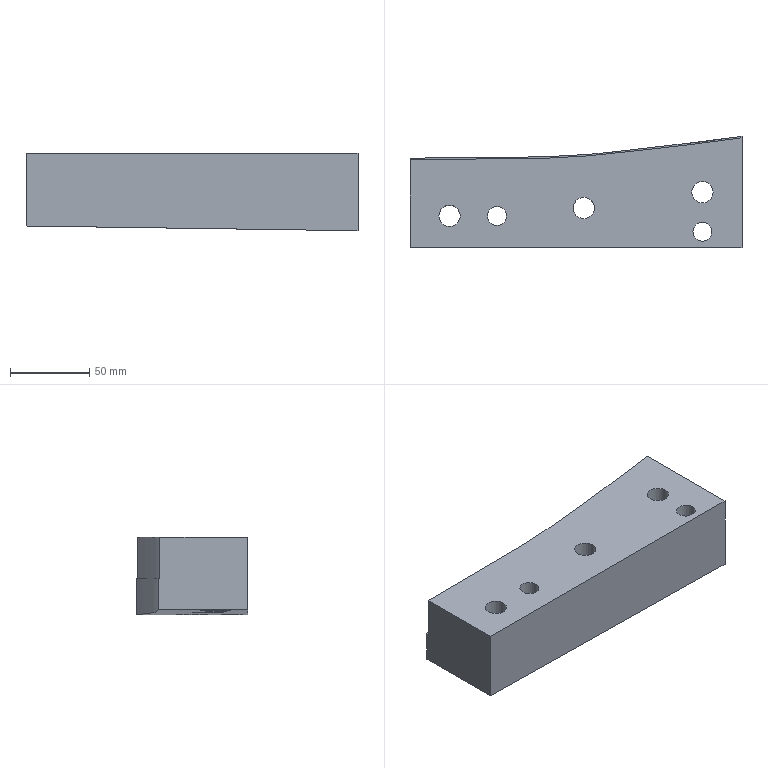Part | NX | features solid 2 | 1 solid | 23 faces | box 210 x 70.368 x 49 mm | volume 559082 mm3 | plane 11 | cylinder 10 | spline 2 | commonest cylinder face diameters 13.5 x3 19.5 x3 12 x2 13 x2
STEP:
#1=CARTESIAN_POINT('',(140.,-80.642,14.));
#2=VERTEX_POINT('',#1);
#3=CARTESIAN_POINT('',(140.,-79.632,14.));
#4=VERTEX_POINT('',#3);
#5=CARTESIAN_POINT('',(140.,-115.282,14.));
#6=DIRECTION('',(0.,1.,0.));
#7=VECTOR('',#6,1000.);
#8=LINE('',#5,#7);
#9=EDGE_CURVE('',#2,#4,#8,.T.);
#10=ORIENTED_EDGE('',*,*,#9,.F.);
#11=CARTESIAN_POINT('',(140.,-80.642,40.));
#12=VERTEX_POINT('',#11);
#13=CARTESIAN_POINT('',(140.,-80.642,57.));
#14=DIRECTION('',(0.,0.,1.));
#15=VECTOR('',#14,1000.);
#16=LINE('',#13,#15);
#17=EDGE_CURVE('',#12,#2,#16,.F.);
#18=ORIENTED_EDGE('',*,*,#17,.F.);
#19=CARTESIAN_POINT('',(140.,-150.,40.));
#20=VERTEX_POINT('',#19);
#21=CARTESIAN_POINT('',(140.,35.09,40.));
#22=DIRECTION('',(0.,1.,0.));
#23=VECTOR('',#22,1000.);
#24=LINE('',#21,#23);
#25=EDGE_CURVE('',#20,#12,#24,.T.);
#26=ORIENTED_EDGE('',*,*,#25,.F.);
#27=CARTESIAN_POINT('',(140.,-150.,-9.));
#28=VERTEX_POINT('',#27);
#29=CARTESIAN_POINT('',(140.,-150.,2.));
#30=DIRECTION('',(0.,0.,-1.));
#31=VECTOR('',#30,1000.);
#32=LINE('',#29,#31);
#33=EDGE_CURVE('',#20,#28,#32,.T.);
#34=ORIENTED_EDGE('',*,*,#33,.T.);
#35=CARTESIAN_POINT('',(140.,-79.632,-9.));
#36=VERTEX_POINT('',#35);
#37=CARTESIAN_POINT('',(140.,-222.,-9.));
#38=DIRECTION('',(0.,-1.,0.));
#39=VECTOR('',#38,1000.);
#40=LINE('',#37,#39);
#41=EDGE_CURVE('',#36,#28,#40,.T.);
#42=ORIENTED_EDGE('',*,*,#41,.F.);
#43=CARTESIAN_POINT('',(140.,-79.632,27.));
#44=DIRECTION('',(0.,0.,-1.));
#45=VECTOR('',#44,1000.);
#46=LINE('',#43,#45);
#47=EDGE_CURVE('',#4,#36,#46,.T.);
#48=ORIENTED_EDGE('',*,*,#47,.F.);
#49=EDGE_LOOP('',(#10,#18,#26,#34,#42,#48));
#50=FACE_BOUND('',#49,.T.);
#51=CARTESIAN_POINT('',(140.,-115.282,21.5));
#52=DIRECTION('',(1.,0.,0.));
#53=DIRECTION('',(0.,0.,-1.));
#54=AXIS2_PLACEMENT_3D('',#51,#52,#53);
#55=PLANE('',#54);
#56=ADVANCED_FACE('',(#50),#55,.T.);
#57=CARTESIAN_POINT('',(-70.,-93.417,14.));
#58=VERTEX_POINT('',#57);
#59=CARTESIAN_POINT('',(-70.,-94.417,14.));
#60=VERTEX_POINT('',#59);
#61=CARTESIAN_POINT('',(-70.,-99.381,14.));
#62=DIRECTION('',(0.,-1.,0.));
#63=VECTOR('',#62,1000.);
#64=LINE('',#61,#63);
#65=EDGE_CURVE('',#58,#60,#64,.T.);
#66=ORIENTED_EDGE('',*,*,#65,.F.);
#67=CARTESIAN_POINT('',(-70.,-93.417,-6.));
#68=VERTEX_POINT('',#67);
#69=CARTESIAN_POINT('',(-70.,-93.417,27.));
#70=DIRECTION('',(0.,0.,-1.));
#71=VECTOR('',#70,1000.);
#72=LINE('',#69,#71);
#73=EDGE_CURVE('',#58,#68,#72,.T.);
#74=ORIENTED_EDGE('',*,*,#73,.T.);
#75=CARTESIAN_POINT('',(-70.,-150.,-6.));
#76=VERTEX_POINT('',#75);
#77=CARTESIAN_POINT('',(-70.,-99.381,-6.));
#78=DIRECTION('',(0.,-1.,0.));
#79=VECTOR('',#78,1000.);
#80=LINE('',#77,#79);
#81=EDGE_CURVE('',#68,#76,#80,.T.);
#82=ORIENTED_EDGE('',*,*,#81,.T.);
#83=CARTESIAN_POINT('',(-70.,-150.,40.));
#84=VERTEX_POINT('',#83);
#85=CARTESIAN_POINT('',(-70.,-150.,-66.));
#86=DIRECTION('',(0.,0.,-1.));
#87=VECTOR('',#86,1000.);
#88=LINE('',#85,#87);
#89=EDGE_CURVE('',#84,#76,#88,.T.);
#90=ORIENTED_EDGE('',*,*,#89,.F.);
#91=CARTESIAN_POINT('',(-70.,-94.417,40.));
#92=VERTEX_POINT('',#91);
#93=CARTESIAN_POINT('',(-70.,35.09,40.));
#94=DIRECTION('',(0.,-1.,0.));
#95=VECTOR('',#94,1000.);
#96=LINE('',#93,#95);
#97=EDGE_CURVE('',#92,#84,#96,.T.);
#98=ORIENTED_EDGE('',*,*,#97,.F.);
#99=CARTESIAN_POINT('',(-70.,-94.417,57.));
#100=DIRECTION('',(0.,0.,1.));
#101=VECTOR('',#100,1000.);
#102=LINE('',#99,#101);
#103=EDGE_CURVE('',#60,#92,#102,.T.);
#104=ORIENTED_EDGE('',*,*,#103,.F.);
#105=EDGE_LOOP('',(#66,#74,#82,#90,#98,#104));
#106=FACE_BOUND('',#105,.T.);
#107=CARTESIAN_POINT('',(-70.,-99.381,-66.));
#108=DIRECTION('',(-1.,0.,0.));
#109=DIRECTION('',(0.,0.,1.));
#110=AXIS2_PLACEMENT_3D('',#107,#108,#109);
#111=PLANE('',#110);
#112=ADVANCED_FACE('',(#106),#111,.T.);
#113=CARTESIAN_POINT('',(-190.231,-121.49,14.));
#114=CARTESIAN_POINT('',(-188.654,-121.152,14.));
#115=CARTESIAN_POINT('',(-185.47,-120.627,14.));
#116=CARTESIAN_POINT('',(-180.656,-120.141,14.));
#117=CARTESIAN_POINT('',(-175.882,-119.326,14.));
#118=CARTESIAN_POINT('',(-169.679,-117.528,14.));
#119=CARTESIAN_POINT('',(-162.185,-114.539,14.));
#120=CARTESIAN_POINT('',(-153.086,-111.254,14.));
#121=CARTESIAN_POINT('',(-144.031,-107.845,14.));
#122=CARTESIAN_POINT('',(-136.465,-105.061,14.));
#123=CARTESIAN_POINT('',(-130.418,-102.814,14.));
#124=CARTESIAN_POINT('',(-125.812,-101.329,14.));
#125=CARTESIAN_POINT('',(-121.306,-99.566,14.));
#126=CARTESIAN_POINT('',(-116.876,-97.626,14.));
#127=CARTESIAN_POINT('',(-112.335,-95.923,14.));
#128=CARTESIAN_POINT('',(-107.564,-95.05,14.));
#129=CARTESIAN_POINT('',(-102.756,-94.525,14.));
#130=CARTESIAN_POINT('',(-96.349,-93.771,14.));
#131=CARTESIAN_POINT('',(-89.902,-93.468,14.));
#132=CARTESIAN_POINT('',(-83.452,-93.448,14.));
#133=CARTESIAN_POINT('',(-77.002,-93.469,14.));
#134=CARTESIAN_POINT('',(-68.939,-93.411,14.));
#135=CARTESIAN_POINT('',(-56.04,-93.3,14.));
#136=CARTESIAN_POINT('',(-33.465,-93.184,14.));
#137=CARTESIAN_POINT('',(-7.666,-93.074,14.));
#138=CARTESIAN_POINT('',(14.907,-92.653,14.));
#139=CARTESIAN_POINT('',(27.794,-92.068,14.));
#140=CARTESIAN_POINT('',(40.668,-91.245,14.));
#141=CARTESIAN_POINT('',(51.917,-90.291,14.));
#142=CARTESIAN_POINT('',(61.528,-89.174,14.));
#143=CARTESIAN_POINT('',(67.939,-88.466,14.));
#144=CARTESIAN_POINT('',(79.125,-86.95,14.));
#145=CARTESIAN_POINT('',(95.161,-85.253,14.));
#146=CARTESIAN_POINT('',(114.404,-83.21,14.));
#147=CARTESIAN_POINT('',(133.568,-80.524,14.));
#148=CARTESIAN_POINT('',(152.734,-77.861,14.));
#149=CARTESIAN_POINT('',(171.916,-75.326,14.));
#150=CARTESIAN_POINT('',(191.055,-72.413,14.));
#151=CARTESIAN_POINT('',(207.17,-71.468,14.));
#152=CARTESIAN_POINT('',(219.951,-69.697,14.));
#153=CARTESIAN_POINT('',(232.724,-67.899,14.));
#154=CARTESIAN_POINT('',(248.708,-65.766,14.));
#155=CARTESIAN_POINT('',(267.87,-63.074,14.));
#156=CARTESIAN_POINT('',(287.038,-60.44,14.));
#157=CARTESIAN_POINT('',(301.448,-58.682,14.));
#158=CARTESIAN_POINT('',(310.976,-56.987,14.));
#159=CARTESIAN_POINT('',(314.916,-56.135,14.));
#160=CARTESIAN_POINT('',(318.052,-55.382,14.));
#161=CARTESIAN_POINT('',(320.39,-54.76,14.));
#162=CARTESIAN_POINT('',(322.686,-53.981,14.));
#163=CARTESIAN_POINT('',(325.595,-52.578,14.));
#164=CARTESIAN_POINT('',(328.769,-50.098,14.));
#165=CARTESIAN_POINT('',(332.247,-46.69,14.));
#166=CARTESIAN_POINT('',(335.795,-43.406,14.));
#167=CARTESIAN_POINT('',(343.661,-37.758,14.));
#168=CARTESIAN_POINT('',(355.164,-28.914,14.));
#169=CARTESIAN_POINT('',(370.422,-17.018,14.));
#170=CARTESIAN_POINT('',(383.264,-7.249,14.));
#171=CARTESIAN_POINT('',(392.416,-0.6713,14.));
#172=CARTESIAN_POINT('',(396.953,2.733,14.));
#173=CARTESIAN_POINT('',(398.886,5.372,14.));
#174=CARTESIAN_POINT('',(399.725,7.654,14.));
#175=CARTESIAN_POINT('',(399.76,10.078,14.));
#176=CARTESIAN_POINT('',(399.483,13.317,14.));
#177=CARTESIAN_POINT('',(399.712,17.34,14.));
#178=CARTESIAN_POINT('',(399.612,22.179,14.));
#179=CARTESIAN_POINT('',(399.633,31.854,14.));
#180=CARTESIAN_POINT('',(399.593,46.366,14.));
#181=CARTESIAN_POINT('',(399.637,62.491,14.));
#182=CARTESIAN_POINT('',(399.588,73.779,14.));
#183=CARTESIAN_POINT('',(399.652,79.422,14.));
#184=CARTESIAN_POINT('',(399.59,82.647,14.));
#185=CARTESIAN_POINT('',(399.564,85.065,14.));
#186=CARTESIAN_POINT('',(399.725,87.486,14.));
#187=CARTESIAN_POINT('',(399.756,89.902,14.));
#188=CARTESIAN_POINT('',(399.247,92.301,14.));
#189=CARTESIAN_POINT('',(397.362,95.008,14.));
#190=CARTESIAN_POINT('',(393.635,96.774,14.));
#191=CARTESIAN_POINT('',(389.279,98.826,14.));
#192=CARTESIAN_POINT('',(384.732,100.498,14.));
#193=CARTESIAN_POINT('',(378.765,102.95,14.));
#194=CARTESIAN_POINT('',(362.589,110.229,14.));
#195=CARTESIAN_POINT('',(344.928,118.135,14.));
#196=CARTESIAN_POINT('',(327.281,126.072,14.));
#197=CARTESIAN_POINT('',(319.932,129.381,14.));
#198=CARTESIAN_POINT('',(314.075,132.102,14.));
#199=CARTESIAN_POINT('',(309.387,133.376,14.));
#200=CARTESIAN_POINT('',(304.547,133.785,14.));
#201=CARTESIAN_POINT('',(299.716,133.401,14.));
#202=CARTESIAN_POINT('',(294.929,132.704,14.));
#203=CARTESIAN_POINT('',(288.543,131.8,14.));
#204=CARTESIAN_POINT('',(277.364,130.241,14.));
#205=CARTESIAN_POINT('',(242.2,125.552,14.));
#206=CARTESIAN_POINT('',(184.637,118.048,14.));
#207=CARTESIAN_POINT('',(120.701,109.541,14.));
#208=CARTESIAN_POINT('',(69.531,102.902,14.));
#209=CARTESIAN_POINT('',(40.777,98.94,14.));
#210=CARTESIAN_POINT('',(21.566,96.615,14.));
#211=CARTESIAN_POINT('',(8.743,95.212,14.));
#212=CARTESIAN_POINT('',(-7.301,93.575,14.));
#213=CARTESIAN_POINT('',(-26.625,92.505,14.));
#214=CARTESIAN_POINT('',(-45.971,92.017,14.));
#215=CARTESIAN_POINT('',(-62.09,91.675,14.));
#216=CARTESIAN_POINT('',(-74.987,91.256,14.));
#217=CARTESIAN_POINT('',(-84.664,91.165,14.));
#218=CARTESIAN_POINT('',(-94.319,91.781,14.));
#219=CARTESIAN_POINT('',(-103.929,92.966,14.));
#220=CARTESIAN_POINT('',(-113.495,94.403,14.));
#221=CARTESIAN_POINT('',(-119.856,95.492,14.));
#222=CARTESIAN_POINT('',(-122.997,96.222,14.));
#223=B_SPLINE_CURVE_WITH_KNOTS('',3,(#113,#114,#115,#116,#117,#118,#119,#120,#121,#122,#123,#124,#125,#126,#127,#128,#129,#130,#131,#132,#133,#134,#135,#136,#137,#138,#139,#140,#141,#142,#143,#144,#145,#146,#147,#148,#149,#150,#151,#152,#153,#154,#155,#156,#157,#158,#159,#160,#161,#162,#163,#164,#165,#166,#167,#168,#169,#170,#171,#172,#173,#174,#175,#176,#177,#178,#179,#180,#181,#182,#183,#184,#185,#186,#187,#188,#189,#190,#191,#192,#193,#194,#195,#196,#197,#198,#199,#200,#201,#202,#203,#204,#205,#206,#207,#208,#209,#210,#211,#212,#213,#214,#215,#216,#217,#218,#219,#220,#221,#222),.UNSPECIFIED.,.F.,.F.,(4,1,1,1,1,1,1,1,1,1,1,1,1,1,1,1,1,1,1,1,1,1,1,1,1,1,1,1,1,1,1,1,1,1,1,1,1,1,1,1,1,1,1,1,1,1,1,1,1,1,1,1,1,1,1,1,1,1,1,1,1,1,1,1,1,1,1,1,1,1,1,1,1,1,1,1,1,1,1,1,1,1,1,1,1,1,1,1,1,1,1,1,1,1,1,1,1,1,1,1,1,1,1,1,1,1,1,4),(0.4704,0.4724,0.4745,0.4766,0.4786,0.4828,0.4869,0.491,0.4952,0.4972,0.4993,0.5014,0.5035,0.5055,0.5076,0.5097,0.5117,0.5159,0.5179,0.52,0.5241,0.5283,0.5366,0.5531,0.5614,0.5655,0.5697,0.5779,0.58,0.5821,0.5862,0.5945,0.6028,0.611,0.6193,0.6276,0.6359,0.6441,0.6483,0.6524,0.6607,0.669,0.6772,0.6855,0.6876,0.6897,0.6907,0.6917,0.6928,0.6938,0.6959,0.6979,0.7,0.7021,0.7103,0.7186,0.7269,0.731,0.7331,0.7341,0.7352,0.7362,0.7372,0.7393,0.7414,0.7435,0.7517,0.76,0.7641,0.7662,0.7672,0.7683,0.7693,0.7703,0.7714,0.7724,0.7745,0.7766,0.7786,0.7807,0.7848,0.8014,0.8055,0.8097,0.8117,0.8138,0.8159,0.8179,0.82,0.8221,0.8262,0.8345,0.8676,0.9007,0.9172,0.9338,0.9379,0.9421,0.9503,0.9586,0.9669,0.9752,0.9793,0.9834,0.9876,0.9917,0.9959,1.),.UNSPECIFIED.);
#224=EDGE_CURVE('',#4,#58,#223,.F.);
#225=ORIENTED_EDGE('',*,*,#224,.F.);
#226=ORIENTED_EDGE('',*,*,#47,.T.);
#227=CARTESIAN_POINT('',(140.,-79.632,-9.));
#228=CARTESIAN_POINT('',(131.311,-80.839,-8.876));
#229=CARTESIAN_POINT('',(113.944,-83.357,-8.628));
#230=CARTESIAN_POINT('',(92.136,-85.521,-8.316));
#231=CARTESIAN_POINT('',(76.894,-87.264,-8.098));
#232=CARTESIAN_POINT('',(68.201,-88.424,-7.974));
#233=CARTESIAN_POINT('',(59.49,-89.412,-7.85));
#234=CARTESIAN_POINT('',(48.597,-90.606,-7.694));
#235=CARTESIAN_POINT('',(31.113,-91.951,-7.444));
#236=CARTESIAN_POINT('',(9.179,-92.893,-7.131));
#237=CARTESIAN_POINT('',(-26.014,-93.171,-6.628));
#238=CARTESIAN_POINT('',(-52.407,-93.281,-6.251));
#239=CARTESIAN_POINT('',(-70.,-93.417,-6.));
#240=B_SPLINE_CURVE_WITH_KNOTS('',3,(#227,#228,#229,#230,#231,#232,#233,#234,#235,#236,#237,#238,#239),.UNSPECIFIED.,.F.,.F.,(4,1,1,1,1,1,1,1,1,1,4),(0.,0.0263,0.0526,0.06575,0.07233,0.0789,0.09205,0.1052,0.1315,0.1578,0.2104),.UNSPECIFIED.);
#241=EDGE_CURVE('',#36,#68,#240,.T.);
#242=ORIENTED_EDGE('',*,*,#241,.T.);
#243=ORIENTED_EDGE('',*,*,#73,.F.);
#244=EDGE_LOOP('',(#225,#226,#242,#243));
#245=FACE_BOUND('',#244,.T.);
#246=CARTESIAN_POINT('',(-70.,-93.417,14.));
#247=CARTESIAN_POINT('',(-70.,-93.417,-9.138));
#248=CARTESIAN_POINT('',(-52.44,-93.282,14.));
#249=CARTESIAN_POINT('',(-52.44,-93.282,-9.138));
#250=CARTESIAN_POINT('',(-26.1,-93.171,14.));
#251=CARTESIAN_POINT('',(-26.1,-93.171,-9.138));
#252=CARTESIAN_POINT('',(9.024,-92.895,14.));
#253=CARTESIAN_POINT('',(9.024,-92.895,-9.138));
#254=CARTESIAN_POINT('',(30.956,-91.96,14.));
#255=CARTESIAN_POINT('',(30.956,-91.96,-9.138));
#256=CARTESIAN_POINT('',(48.469,-90.618,14.));
#257=CARTESIAN_POINT('',(48.469,-90.618,-9.138));
#258=CARTESIAN_POINT('',(59.38,-89.424,14.));
#259=CARTESIAN_POINT('',(59.38,-89.424,-9.138));
#260=CARTESIAN_POINT('',(68.104,-88.436,14.));
#261=CARTESIAN_POINT('',(68.104,-88.436,-9.138));
#262=CARTESIAN_POINT('',(76.808,-87.275,14.));
#263=CARTESIAN_POINT('',(76.808,-87.275,-9.138));
#264=CARTESIAN_POINT('',(92.073,-85.527,14.));
#265=CARTESIAN_POINT('',(92.073,-85.527,-9.138));
#266=CARTESIAN_POINT('',(113.921,-83.361,14.));
#267=CARTESIAN_POINT('',(113.921,-83.361,-9.138));
#268=CARTESIAN_POINT('',(131.303,-80.84,14.));
#269=CARTESIAN_POINT('',(131.303,-80.84,-9.138));
#270=CARTESIAN_POINT('',(140.,-79.632,14.));
#271=CARTESIAN_POINT('',(140.,-79.632,-9.138));
#272=B_SPLINE_SURFACE_WITH_KNOTS('',3,1,((#246,#247),(#248,#249),(#250,#251),(#252,#253),(#254,#255),(#256,#257),(#258,#259),(#260,#261),(#262,#263),(#264,#265),(#266,#267),(#268,#269),(#270,#271)),.SURF_OF_LINEAR_EXTRUSION.,.F.,.F.,.F.,(4,1,1,1,1,1,1,1,1,1,4),(2,2),(0.5237,0.5462,0.5575,0.5688,0.5744,0.58,0.5828,0.5857,0.5913,0.6026,0.6138),(0.,1.),.UNSPECIFIED.);
#273=ADVANCED_FACE('',(#245),#272,.T.);
#274=ORIENTED_EDGE('',*,*,#33,.F.);
#275=CARTESIAN_POINT('',(-415.478,-150.,40.));
#276=DIRECTION('',(-1.,0.,0.));
#277=VECTOR('',#276,1000.);
#278=LINE('',#275,#277);
#279=EDGE_CURVE('',#20,#84,#278,.T.);
#280=ORIENTED_EDGE('',*,*,#279,.T.);
#281=ORIENTED_EDGE('',*,*,#89,.T.);
#282=CARTESIAN_POINT('',(-470.299,-150.,-0.2814));
#283=DIRECTION('',(-0.9999,0.,0.01428));
#284=VECTOR('',#283,1000.);
#285=LINE('',#282,#284);
#286=EDGE_CURVE('',#28,#76,#285,.T.);
#287=ORIENTED_EDGE('',*,*,#286,.F.);
#288=EDGE_LOOP('',(#274,#280,#281,#287));
#289=FACE_BOUND('',#288,.T.);
#290=CARTESIAN_POINT('',(0.,-150.,2.));
#291=DIRECTION('',(0.,1.,0.));
#292=DIRECTION('',(0.,0.,1.));
#293=AXIS2_PLACEMENT_3D('',#290,#291,#292);
#294=PLANE('',#293);
#295=ADVANCED_FACE('',(#289),#294,.F.);
#296=CARTESIAN_POINT('',(-70.,-94.417,40.));
#297=CARTESIAN_POINT('',(-52.434,-94.282,40.));
#298=CARTESIAN_POINT('',(-26.078,-94.171,40.));
#299=CARTESIAN_POINT('',(9.055,-93.894,40.));
#300=CARTESIAN_POINT('',(30.962,-92.961,40.));
#301=CARTESIAN_POINT('',(48.45,-91.624,40.));
#302=CARTESIAN_POINT('',(59.356,-90.433,40.));
#303=CARTESIAN_POINT('',(68.079,-89.447,40.));
#304=CARTESIAN_POINT('',(76.791,-88.286,40.));
#305=CARTESIAN_POINT('',(92.054,-86.532,40.));
#306=CARTESIAN_POINT('',(113.882,-84.374,40.));
#307=CARTESIAN_POINT('',(131.292,-81.851,40.));
#308=CARTESIAN_POINT('',(140.,-80.642,40.));
#309=B_SPLINE_CURVE_WITH_KNOTS('',3,(#296,#297,#298,#299,#300,#301,#302,#303,#304,#305,#306,#307,#308),.UNSPECIFIED.,.F.,.F.,(4,1,1,1,1,1,1,1,1,1,4),(0.,0.05261,0.07892,0.1052,0.1184,0.1315,0.1381,0.1447,0.1578,0.1841,0.2105),.UNSPECIFIED.);
#310=EDGE_CURVE('',#92,#12,#309,.T.);
#311=ORIENTED_EDGE('',*,*,#310,.F.);
#312=ORIENTED_EDGE('',*,*,#97,.T.);
#313=ORIENTED_EDGE('',*,*,#279,.F.);
#314=ORIENTED_EDGE('',*,*,#25,.T.);
#315=EDGE_LOOP('',(#311,#312,#313,#314));
#316=FACE_BOUND('',#315,.T.);
#317=CARTESIAN_POINT('',(121.,-140.,40.));
#318=VERTEX_POINT('',#317);
#319=CARTESIAN_POINT('',(115.,-140.,40.));
#320=DIRECTION('',(0.,0.,1.));
#321=DIRECTION('',(1.,0.,0.));
#322=AXIS2_PLACEMENT_3D('',#319,#320,#321);
#323=CIRCLE('',#322,6.);
#324=EDGE_CURVE('',#318,#318,#323,.T.);
#325=ORIENTED_EDGE('',*,*,#324,.F.);
#326=EDGE_LOOP('',(#325));
#327=FACE_BOUND('',#326,.T.);
#328=CARTESIAN_POINT('',(-9.,-130.,40.));
#329=VERTEX_POINT('',#328);
#330=CARTESIAN_POINT('',(-15.,-130.,40.));
#331=DIRECTION('',(0.,0.,1.));
#332=DIRECTION('',(1.,0.,0.));
#333=AXIS2_PLACEMENT_3D('',#330,#331,#332);
#334=CIRCLE('',#333,6.);
#335=EDGE_CURVE('',#329,#329,#334,.T.);
#336=ORIENTED_EDGE('',*,*,#335,.F.);
#337=EDGE_LOOP('',(#336));
#338=FACE_BOUND('',#337,.T.);
#339=CARTESIAN_POINT('',(46.75,-125.,40.));
#340=VERTEX_POINT('',#339);
#341=CARTESIAN_POINT('',(40.,-125.,40.));
#342=DIRECTION('',(0.,0.,1.));
#343=DIRECTION('',(1.,0.,0.));
#344=AXIS2_PLACEMENT_3D('',#341,#342,#343);
#345=CIRCLE('',#344,6.75);
#346=EDGE_CURVE('',#340,#340,#345,.T.);
#347=ORIENTED_EDGE('',*,*,#346,.F.);
#348=EDGE_LOOP('',(#347));
#349=FACE_BOUND('',#348,.T.);
#350=CARTESIAN_POINT('',(121.75,-115.,40.));
#351=VERTEX_POINT('',#350);
#352=CARTESIAN_POINT('',(115.,-115.,40.));
#353=DIRECTION('',(0.,0.,1.));
#354=DIRECTION('',(1.,0.,0.));
#355=AXIS2_PLACEMENT_3D('',#352,#353,#354);
#356=CIRCLE('',#355,6.75);
#357=EDGE_CURVE('',#351,#351,#356,.T.);
#358=ORIENTED_EDGE('',*,*,#357,.F.);
#359=EDGE_LOOP('',(#358));
#360=FACE_BOUND('',#359,.T.);
#361=CARTESIAN_POINT('',(-38.25,-130.,40.));
#362=VERTEX_POINT('',#361);
#363=CARTESIAN_POINT('',(-45.,-130.,40.));
#364=DIRECTION('',(0.,0.,1.));
#365=DIRECTION('',(1.,0.,0.));
#366=AXIS2_PLACEMENT_3D('',#363,#364,#365);
#367=CIRCLE('',#366,6.75);
#368=EDGE_CURVE('',#362,#362,#367,.T.);
#369=ORIENTED_EDGE('',*,*,#368,.F.);
#370=EDGE_LOOP('',(#369));
#371=FACE_BOUND('',#370,.T.);
#372=CARTESIAN_POINT('',(-415.478,35.09,40.));
#373=DIRECTION('',(0.,0.,1.));
#374=DIRECTION('',(1.,0.,0.));
#375=AXIS2_PLACEMENT_3D('',#372,#373,#374);
#376=PLANE('',#375);
#377=ADVANCED_FACE('',(#316,#327,#338,#349,#360,#371),#376,.T.);
#378=ORIENTED_EDGE('',*,*,#368,.T.);
#379=EDGE_LOOP('',(#378));
#380=FACE_BOUND('',#379,.T.);
#381=CARTESIAN_POINT('',(-38.25,-130.,9.));
#382=VERTEX_POINT('',#381);
#383=CARTESIAN_POINT('',(-45.,-130.,9.));
#384=DIRECTION('',(0.,0.,1.));
#385=DIRECTION('',(1.,0.,0.));
#386=AXIS2_PLACEMENT_3D('',#383,#384,#385);
#387=CIRCLE('',#386,6.75);
#388=EDGE_CURVE('',#382,#382,#387,.T.);
#389=ORIENTED_EDGE('',*,*,#388,.F.);
#390=EDGE_LOOP('',(#389));
#391=FACE_BOUND('',#390,.T.);
#392=CARTESIAN_POINT('',(-45.,-130.,94.));
#393=DIRECTION('',(0.,0.,1.));
#394=DIRECTION('',(1.,0.,0.));
#395=AXIS2_PLACEMENT_3D('',#392,#393,#394);
#396=CYLINDRICAL_SURFACE('',#395,6.75);
#397=ADVANCED_FACE('',(#380,#391),#396,.F.);
#398=ORIENTED_EDGE('',*,*,#388,.T.);
#399=EDGE_LOOP('',(#398));
#400=FACE_BOUND('',#399,.T.);
#401=CARTESIAN_POINT('',(-35.25,-130.,9.));
#402=VERTEX_POINT('',#401);
#403=CARTESIAN_POINT('',(-45.,-130.,9.));
#404=DIRECTION('',(0.,0.,1.));
#405=DIRECTION('',(1.,0.,0.));
#406=AXIS2_PLACEMENT_3D('',#403,#404,#405);
#407=CIRCLE('',#406,9.75);
#408=EDGE_CURVE('',#402,#402,#407,.T.);
#409=ORIENTED_EDGE('',*,*,#408,.F.);
#410=EDGE_LOOP('',(#409));
#411=FACE_BOUND('',#410,.T.);
#412=CARTESIAN_POINT('',(-45.,-130.,9.));
#413=DIRECTION('',(0.,0.,1.));
#414=DIRECTION('',(1.,0.,0.));
#415=AXIS2_PLACEMENT_3D('',#412,#413,#414);
#416=PLANE('',#415);
#417=ADVANCED_FACE('',(#400,#411),#416,.F.);
#418=ORIENTED_EDGE('',*,*,#408,.T.);
#419=EDGE_LOOP('',(#418));
#420=FACE_BOUND('',#419,.T.);
#421=CARTESIAN_POINT('',(-35.25,-130.,-6.496));
#422=VERTEX_POINT('',#421);
#423=CARTESIAN_POINT('',(-45.,-130.,-6.357));
#424=DIRECTION('',(-0.01428,0.,-0.9999));
#425=DIRECTION('',(0.9999,0.,-0.01428));
#426=AXIS2_PLACEMENT_3D('',#423,#424,#425);
#427=ELLIPSE('',#426,9.751,9.75);
#428=EDGE_CURVE('',#422,#422,#427,.T.);
#429=ORIENTED_EDGE('',*,*,#428,.T.);
#430=EDGE_LOOP('',(#429));
#431=FACE_BOUND('',#430,.T.);
#432=CARTESIAN_POINT('',(-45.,-130.,-6.));
#433=DIRECTION('',(0.,0.,1.));
#434=DIRECTION('',(1.,0.,0.));
#435=AXIS2_PLACEMENT_3D('',#432,#433,#434);
#436=CYLINDRICAL_SURFACE('',#435,9.75);
#437=ADVANCED_FACE('',(#420,#431),#436,.F.);
#438=ORIENTED_EDGE('',*,*,#357,.T.);
#439=EDGE_LOOP('',(#438));
#440=FACE_BOUND('',#439,.T.);
#441=CARTESIAN_POINT('',(121.75,-115.,9.));
#442=VERTEX_POINT('',#441);
#443=CARTESIAN_POINT('',(115.,-115.,9.));
#444=DIRECTION('',(0.,0.,1.));
#445=DIRECTION('',(1.,0.,0.));
#446=AXIS2_PLACEMENT_3D('',#443,#444,#445);
#447=CIRCLE('',#446,6.75);
#448=EDGE_CURVE('',#442,#442,#447,.T.);
#449=ORIENTED_EDGE('',*,*,#448,.F.);
#450=EDGE_LOOP('',(#449));
#451=FACE_BOUND('',#450,.T.);
#452=CARTESIAN_POINT('',(115.,-115.,94.));
#453=DIRECTION('',(0.,0.,1.));
#454=DIRECTION('',(1.,0.,0.));
#455=AXIS2_PLACEMENT_3D('',#452,#453,#454);
#456=CYLINDRICAL_SURFACE('',#455,6.75);
#457=ADVANCED_FACE('',(#440,#451),#456,.F.);
#458=ORIENTED_EDGE('',*,*,#448,.T.);
#459=EDGE_LOOP('',(#458));
#460=FACE_BOUND('',#459,.T.);
#461=CARTESIAN_POINT('',(124.75,-115.,9.));
#462=VERTEX_POINT('',#461);
#463=CARTESIAN_POINT('',(115.,-115.,9.));
#464=DIRECTION('',(0.,0.,1.));
#465=DIRECTION('',(1.,0.,0.));
#466=AXIS2_PLACEMENT_3D('',#463,#464,#465);
#467=CIRCLE('',#466,9.75);
#468=EDGE_CURVE('',#462,#462,#467,.T.);
#469=ORIENTED_EDGE('',*,*,#468,.F.);
#470=EDGE_LOOP('',(#469));
#471=FACE_BOUND('',#470,.T.);
#472=CARTESIAN_POINT('',(115.,-115.,9.));
#473=DIRECTION('',(0.,0.,1.));
#474=DIRECTION('',(1.,0.,0.));
#475=AXIS2_PLACEMENT_3D('',#472,#473,#474);
#476=PLANE('',#475);
#477=ADVANCED_FACE('',(#460,#471),#476,.F.);
#478=ORIENTED_EDGE('',*,*,#468,.T.);
#479=EDGE_LOOP('',(#478));
#480=FACE_BOUND('',#479,.T.);
#481=CARTESIAN_POINT('',(124.75,-115.,-8.782));
#482=VERTEX_POINT('',#481);
#483=CARTESIAN_POINT('',(115.,-115.,-8.643));
#484=DIRECTION('',(-0.01428,0.,-0.9999));
#485=DIRECTION('',(0.9999,0.,-0.01428));
#486=AXIS2_PLACEMENT_3D('',#483,#484,#485);
#487=ELLIPSE('',#486,9.751,9.75);
#488=EDGE_CURVE('',#482,#482,#487,.T.);
#489=ORIENTED_EDGE('',*,*,#488,.T.);
#490=EDGE_LOOP('',(#489));
#491=FACE_BOUND('',#490,.T.);
#492=CARTESIAN_POINT('',(115.,-115.,-6.));
#493=DIRECTION('',(0.,0.,1.));
#494=DIRECTION('',(1.,0.,0.));
#495=AXIS2_PLACEMENT_3D('',#492,#493,#494);
#496=CYLINDRICAL_SURFACE('',#495,9.75);
#497=ADVANCED_FACE('',(#480,#491),#496,.F.);
#498=ORIENTED_EDGE('',*,*,#346,.T.);
#499=EDGE_LOOP('',(#498));
#500=FACE_BOUND('',#499,.T.);
#501=CARTESIAN_POINT('',(46.75,-125.,9.));
#502=VERTEX_POINT('',#501);
#503=CARTESIAN_POINT('',(40.,-125.,9.));
#504=DIRECTION('',(0.,0.,1.));
#505=DIRECTION('',(1.,0.,0.));
#506=AXIS2_PLACEMENT_3D('',#503,#504,#505);
#507=CIRCLE('',#506,6.75);
#508=EDGE_CURVE('',#502,#502,#507,.T.);
#509=ORIENTED_EDGE('',*,*,#508,.F.);
#510=EDGE_LOOP('',(#509));
#511=FACE_BOUND('',#510,.T.);
#512=CARTESIAN_POINT('',(40.,-125.,94.));
#513=DIRECTION('',(0.,0.,1.));
#514=DIRECTION('',(1.,0.,0.));
#515=AXIS2_PLACEMENT_3D('',#512,#513,#514);
#516=CYLINDRICAL_SURFACE('',#515,6.75);
#517=ADVANCED_FACE('',(#500,#511),#516,.F.);
#518=ORIENTED_EDGE('',*,*,#508,.T.);
#519=EDGE_LOOP('',(#518));
#520=FACE_BOUND('',#519,.T.);
#521=CARTESIAN_POINT('',(49.75,-125.,9.));
#522=VERTEX_POINT('',#521);
#523=CARTESIAN_POINT('',(40.,-125.,9.));
#524=DIRECTION('',(0.,0.,1.));
#525=DIRECTION('',(1.,0.,0.));
#526=AXIS2_PLACEMENT_3D('',#523,#524,#525);
#527=CIRCLE('',#526,9.75);
#528=EDGE_CURVE('',#522,#522,#527,.T.);
#529=ORIENTED_EDGE('',*,*,#528,.F.);
#530=EDGE_LOOP('',(#529));
#531=FACE_BOUND('',#530,.T.);
#532=CARTESIAN_POINT('',(40.,-125.,9.));
#533=DIRECTION('',(0.,0.,1.));
#534=DIRECTION('',(1.,0.,0.));
#535=AXIS2_PLACEMENT_3D('',#532,#533,#534);
#536=PLANE('',#535);
#537=ADVANCED_FACE('',(#520,#531),#536,.F.);
#538=ORIENTED_EDGE('',*,*,#528,.T.);
#539=EDGE_LOOP('',(#538));
#540=FACE_BOUND('',#539,.T.);
#541=CARTESIAN_POINT('',(49.75,-125.,-7.711));
#542=VERTEX_POINT('',#541);
#543=CARTESIAN_POINT('',(40.,-125.,-7.571));
#544=DIRECTION('',(-0.01428,0.,-0.9999));
#545=DIRECTION('',(0.9999,0.,-0.01428));
#546=AXIS2_PLACEMENT_3D('',#543,#544,#545);
#547=ELLIPSE('',#546,9.751,9.75);
#548=EDGE_CURVE('',#542,#542,#547,.T.);
#549=ORIENTED_EDGE('',*,*,#548,.T.);
#550=EDGE_LOOP('',(#549));
#551=FACE_BOUND('',#550,.T.);
#552=CARTESIAN_POINT('',(40.,-125.,-6.));
#553=DIRECTION('',(0.,0.,1.));
#554=DIRECTION('',(1.,0.,0.));
#555=AXIS2_PLACEMENT_3D('',#552,#553,#554);
#556=CYLINDRICAL_SURFACE('',#555,9.75);
#557=ADVANCED_FACE('',(#540,#551),#556,.F.);
#558=ORIENTED_EDGE('',*,*,#335,.T.);
#559=EDGE_LOOP('',(#558));
#560=FACE_BOUND('',#559,.T.);
#561=CARTESIAN_POINT('',(-9.,-130.,14.));
#562=VERTEX_POINT('',#561);
#563=CARTESIAN_POINT('',(-15.,-130.,14.));
#564=DIRECTION('',(0.,0.,1.));
#565=DIRECTION('',(1.,0.,0.));
#566=AXIS2_PLACEMENT_3D('',#563,#564,#565);
#567=CIRCLE('',#566,6.);
#568=EDGE_CURVE('',#562,#562,#567,.T.);
#569=ORIENTED_EDGE('',*,*,#568,.F.);
#570=EDGE_LOOP('',(#569));
#571=FACE_BOUND('',#570,.T.);
#572=CARTESIAN_POINT('',(-15.,-130.,94.));
#573=DIRECTION('',(0.,0.,1.));
#574=DIRECTION('',(1.,0.,0.));
#575=AXIS2_PLACEMENT_3D('',#572,#573,#574);
#576=CYLINDRICAL_SURFACE('',#575,6.);
#577=ADVANCED_FACE('',(#560,#571),#576,.F.);
#578=ORIENTED_EDGE('',*,*,#568,.T.);
#579=EDGE_LOOP('',(#578));
#580=FACE_BOUND('',#579,.T.);
#581=CARTESIAN_POINT('',(-8.5,-130.,14.));
#582=VERTEX_POINT('',#581);
#583=CARTESIAN_POINT('',(-15.,-130.,14.));
#584=DIRECTION('',(0.,0.,1.));
#585=DIRECTION('',(1.,0.,0.));
#586=AXIS2_PLACEMENT_3D('',#583,#584,#585);
#587=CIRCLE('',#586,6.5);
#588=EDGE_CURVE('',#582,#582,#587,.T.);
#589=ORIENTED_EDGE('',*,*,#588,.F.);
#590=EDGE_LOOP('',(#589));
#591=FACE_BOUND('',#590,.T.);
#592=CARTESIAN_POINT('',(-15.,-130.,14.));
#593=DIRECTION('',(0.,0.,1.));
#594=DIRECTION('',(1.,0.,0.));
#595=AXIS2_PLACEMENT_3D('',#592,#593,#594);
#596=PLANE('',#595);
#597=ADVANCED_FACE('',(#580,#591),#596,.F.);
#598=ORIENTED_EDGE('',*,*,#588,.T.);
#599=EDGE_LOOP('',(#598));
#600=FACE_BOUND('',#599,.T.);
#601=CARTESIAN_POINT('',(-8.5,-130.,-6.879));
#602=VERTEX_POINT('',#601);
#603=CARTESIAN_POINT('',(-15.,-130.,-6.786));
#604=DIRECTION('',(-0.01428,0.,-0.9999));
#605=DIRECTION('',(0.9999,0.,-0.01428));
#606=AXIS2_PLACEMENT_3D('',#603,#604,#605);
#607=ELLIPSE('',#606,6.501,6.5);
#608=EDGE_CURVE('',#602,#602,#607,.T.);
#609=ORIENTED_EDGE('',*,*,#608,.T.);
#610=EDGE_LOOP('',(#609));
#611=FACE_BOUND('',#610,.T.);
#612=CARTESIAN_POINT('',(-15.,-130.,-6.));
#613=DIRECTION('',(0.,0.,1.));
#614=DIRECTION('',(1.,0.,0.));
#615=AXIS2_PLACEMENT_3D('',#612,#613,#614);
#616=CYLINDRICAL_SURFACE('',#615,6.5);
#617=ADVANCED_FACE('',(#600,#611),#616,.F.);
#618=ORIENTED_EDGE('',*,*,#324,.T.);
#619=EDGE_LOOP('',(#618));
#620=FACE_BOUND('',#619,.T.);
#621=CARTESIAN_POINT('',(121.,-140.,14.));
#622=VERTEX_POINT('',#621);
#623=CARTESIAN_POINT('',(115.,-140.,14.));
#624=DIRECTION('',(0.,0.,1.));
#625=DIRECTION('',(1.,0.,0.));
#626=AXIS2_PLACEMENT_3D('',#623,#624,#625);
#627=CIRCLE('',#626,6.);
#628=EDGE_CURVE('',#622,#622,#627,.T.);
#629=ORIENTED_EDGE('',*,*,#628,.F.);
#630=EDGE_LOOP('',(#629));
#631=FACE_BOUND('',#630,.T.);
#632=CARTESIAN_POINT('',(115.,-140.,94.));
#633=DIRECTION('',(0.,0.,1.));
#634=DIRECTION('',(1.,0.,0.));
#635=AXIS2_PLACEMENT_3D('',#632,#633,#634);
#636=CYLINDRICAL_SURFACE('',#635,6.);
#637=ADVANCED_FACE('',(#620,#631),#636,.F.);
#638=ORIENTED_EDGE('',*,*,#628,.T.);
#639=EDGE_LOOP('',(#638));
#640=FACE_BOUND('',#639,.T.);
#641=CARTESIAN_POINT('',(121.5,-140.,14.));
#642=VERTEX_POINT('',#641);
#643=CARTESIAN_POINT('',(115.,-140.,14.));
#644=DIRECTION('',(0.,0.,1.));
#645=DIRECTION('',(1.,0.,0.));
#646=AXIS2_PLACEMENT_3D('',#643,#644,#645);
#647=CIRCLE('',#646,6.5);
#648=EDGE_CURVE('',#642,#642,#647,.T.);
#649=ORIENTED_EDGE('',*,*,#648,.F.);
#650=EDGE_LOOP('',(#649));
#651=FACE_BOUND('',#650,.T.);
#652=CARTESIAN_POINT('',(115.,-140.,14.));
#653=DIRECTION('',(0.,0.,1.));
#654=DIRECTION('',(1.,0.,0.));
#655=AXIS2_PLACEMENT_3D('',#652,#653,#654);
#656=PLANE('',#655);
#657=ADVANCED_FACE('',(#640,#651),#656,.F.);
#658=ORIENTED_EDGE('',*,*,#648,.T.);
#659=EDGE_LOOP('',(#658));
#660=FACE_BOUND('',#659,.T.);
#661=CARTESIAN_POINT('',(121.5,-140.,-8.736));
#662=VERTEX_POINT('',#661);
#663=CARTESIAN_POINT('',(115.,-140.,-8.643));
#664=DIRECTION('',(-0.01428,0.,-0.9999));
#665=DIRECTION('',(0.9999,0.,-0.01428));
#666=AXIS2_PLACEMENT_3D('',#663,#664,#665);
#667=ELLIPSE('',#666,6.501,6.5);
#668=EDGE_CURVE('',#662,#662,#667,.T.);
#669=ORIENTED_EDGE('',*,*,#668,.T.);
#670=EDGE_LOOP('',(#669));
#671=FACE_BOUND('',#670,.T.);
#672=CARTESIAN_POINT('',(115.,-140.,-6.));
#673=DIRECTION('',(0.,0.,1.));
#674=DIRECTION('',(1.,0.,0.));
#675=AXIS2_PLACEMENT_3D('',#672,#673,#674);
#676=CYLINDRICAL_SURFACE('',#675,6.5);
#677=ADVANCED_FACE('',(#660,#671),#676,.F.);
#678=ORIENTED_EDGE('',*,*,#428,.F.);
#679=EDGE_LOOP('',(#678));
#680=FACE_BOUND('',#679,.T.);
#681=ORIENTED_EDGE('',*,*,#488,.F.);
#682=EDGE_LOOP('',(#681));
#683=FACE_BOUND('',#682,.T.);
#684=ORIENTED_EDGE('',*,*,#548,.F.);
#685=EDGE_LOOP('',(#684));
#686=FACE_BOUND('',#685,.T.);
#687=ORIENTED_EDGE('',*,*,#608,.F.);
#688=EDGE_LOOP('',(#687));
#689=FACE_BOUND('',#688,.T.);
#690=ORIENTED_EDGE('',*,*,#668,.F.);
#691=EDGE_LOOP('',(#690));
#692=FACE_BOUND('',#691,.T.);
#693=ORIENTED_EDGE('',*,*,#241,.F.);
#694=ORIENTED_EDGE('',*,*,#41,.T.);
#695=ORIENTED_EDGE('',*,*,#286,.T.);
#696=ORIENTED_EDGE('',*,*,#81,.F.);
#697=EDGE_LOOP('',(#693,#694,#695,#696));
#698=FACE_BOUND('',#697,.T.);
#699=CARTESIAN_POINT('',(-70.,-150.,-6.));
#700=DIRECTION('',(-0.01428,0.,-0.9999));
#701=DIRECTION('',(-0.9999,0.,0.01428));
#702=AXIS2_PLACEMENT_3D('',#699,#700,#701);
#703=PLANE('',#702);
#704=ADVANCED_FACE('',(#680,#683,#686,#689,#692,#698),#703,.T.);
#705=ORIENTED_EDGE('',*,*,#9,.T.);
#706=ORIENTED_EDGE('',*,*,#224,.T.);
#707=ORIENTED_EDGE('',*,*,#65,.T.);
#708=CARTESIAN_POINT('',(-70.,-94.417,14.));
#709=CARTESIAN_POINT('',(-52.446,-94.282,14.));
#710=CARTESIAN_POINT('',(-26.133,-94.171,14.));
#711=CARTESIAN_POINT('',(8.981,-93.896,14.));
#712=CARTESIAN_POINT('',(30.947,-92.963,14.));
#713=CARTESIAN_POINT('',(48.478,-91.621,14.));
#714=CARTESIAN_POINT('',(59.401,-90.428,14.));
#715=CARTESIAN_POINT('',(68.135,-89.44,14.));
#716=CARTESIAN_POINT('',(76.841,-88.28,14.));
#717=CARTESIAN_POINT('',(92.055,-86.533,14.));
#718=CARTESIAN_POINT('',(113.924,-84.368,14.));
#719=CARTESIAN_POINT('',(131.31,-81.849,14.));
#720=CARTESIAN_POINT('',(140.,-80.642,14.));
#721=B_SPLINE_CURVE_WITH_KNOTS('',3,(#708,#709,#710,#711,#712,#713,#714,#715,#716,#717,#718,#719,#720),.UNSPECIFIED.,.F.,.F.,(4,1,1,1,1,1,1,1,1,1,4),(0.5237,0.5462,0.5575,0.5687,0.5744,0.58,0.5828,0.5856,0.5912,0.6025,0.6138),.UNSPECIFIED.);
#722=EDGE_CURVE('',#60,#2,#721,.T.);
#723=ORIENTED_EDGE('',*,*,#722,.T.);
#724=EDGE_LOOP('',(#705,#706,#707,#723));
#725=FACE_BOUND('',#724,.T.);
#726=CARTESIAN_POINT('',(-190.231,-121.49,14.));
#727=DIRECTION('',(0.,0.,-1.));
#728=DIRECTION('',(-1.,0.,0.));
#729=AXIS2_PLACEMENT_3D('',#726,#727,#728);
#730=PLANE('',#729);
#731=ADVANCED_FACE('',(#725),#730,.F.);
#732=ORIENTED_EDGE('',*,*,#17,.T.);
#733=ORIENTED_EDGE('',*,*,#722,.F.);
#734=ORIENTED_EDGE('',*,*,#103,.T.);
#735=ORIENTED_EDGE('',*,*,#310,.T.);
#736=EDGE_LOOP('',(#732,#733,#734,#735));
#737=FACE_BOUND('',#736,.T.);
#738=CARTESIAN_POINT('',(-70.,-94.417,14.));
#739=CARTESIAN_POINT('',(-70.,-94.417,40.));
#740=CARTESIAN_POINT('',(-52.446,-94.282,14.));
#741=CARTESIAN_POINT('',(-52.446,-94.282,40.));
#742=CARTESIAN_POINT('',(-26.133,-94.171,14.));
#743=CARTESIAN_POINT('',(-26.133,-94.171,40.));
#744=CARTESIAN_POINT('',(8.981,-93.896,14.));
#745=CARTESIAN_POINT('',(8.981,-93.896,40.));
#746=CARTESIAN_POINT('',(30.947,-92.963,14.));
#747=CARTESIAN_POINT('',(30.947,-92.963,40.));
#748=CARTESIAN_POINT('',(48.478,-91.621,14.));
#749=CARTESIAN_POINT('',(48.478,-91.621,40.));
#750=CARTESIAN_POINT('',(59.401,-90.428,14.));
#751=CARTESIAN_POINT('',(59.401,-90.428,40.));
#752=CARTESIAN_POINT('',(68.135,-89.44,14.));
#753=CARTESIAN_POINT('',(68.135,-89.44,40.));
#754=CARTESIAN_POINT('',(76.841,-88.28,14.));
#755=CARTESIAN_POINT('',(76.841,-88.28,40.));
#756=CARTESIAN_POINT('',(92.055,-86.533,14.));
#757=CARTESIAN_POINT('',(92.055,-86.533,40.));
#758=CARTESIAN_POINT('',(113.924,-84.368,14.));
#759=CARTESIAN_POINT('',(113.924,-84.368,40.));
#760=CARTESIAN_POINT('',(131.31,-81.849,14.));
#761=CARTESIAN_POINT('',(131.31,-81.849,40.));
#762=CARTESIAN_POINT('',(140.,-80.642,14.));
#763=CARTESIAN_POINT('',(140.,-80.642,40.));
#764=B_SPLINE_SURFACE_WITH_KNOTS('',3,1,((#738,#739),(#740,#741),(#742,#743),(#744,#745),(#746,#747),(#748,#749),(#750,#751),(#752,#753),(#754,#755),(#756,#757),(#758,#759),(#760,#761),(#762,#763)),.SURF_OF_LINEAR_EXTRUSION.,.F.,.F.,.F.,(4,1,1,1,1,1,1,1,1,1,4),(2,2),(0.5237,0.5462,0.5575,0.5687,0.5744,0.58,0.5828,0.5856,0.5912,0.6025,0.6138),(0.,1.),.UNSPECIFIED.);
#765=ADVANCED_FACE('',(#737),#764,.F.);
#766=CLOSED_SHELL('',(#56,#112,#273,#295,#377,#397,#417,#437,#457,#477,#497,#517,#537,#557,#577,#597,#617,#637,#657,#677,#704,#731,#765));
#767=MANIFOLD_SOLID_BREP('',#766);
#768=(LENGTH_UNIT()NAMED_UNIT(*)SI_UNIT(.MILLI.,.METRE.));
#769=UNCERTAINTY_MEASURE_WITH_UNIT(LENGTH_MEASURE(0.0508),#768,'','');
#770=(NAMED_UNIT(*)PLANE_ANGLE_UNIT()SI_UNIT($,.RADIAN.));
#771=(NAMED_UNIT(*)SI_UNIT($,.STERADIAN.)SOLID_ANGLE_UNIT());
#772=(GEOMETRIC_REPRESENTATION_CONTEXT(3)GLOBAL_UNCERTAINTY_ASSIGNED_CONTEXT((#769))GLOBAL_UNIT_ASSIGNED_CONTEXT((#768,#770,#771))REPRESENTATION_CONTEXT('',''));
#773=ADVANCED_BREP_SHAPE_REPRESENTATION('',(#767),#772);